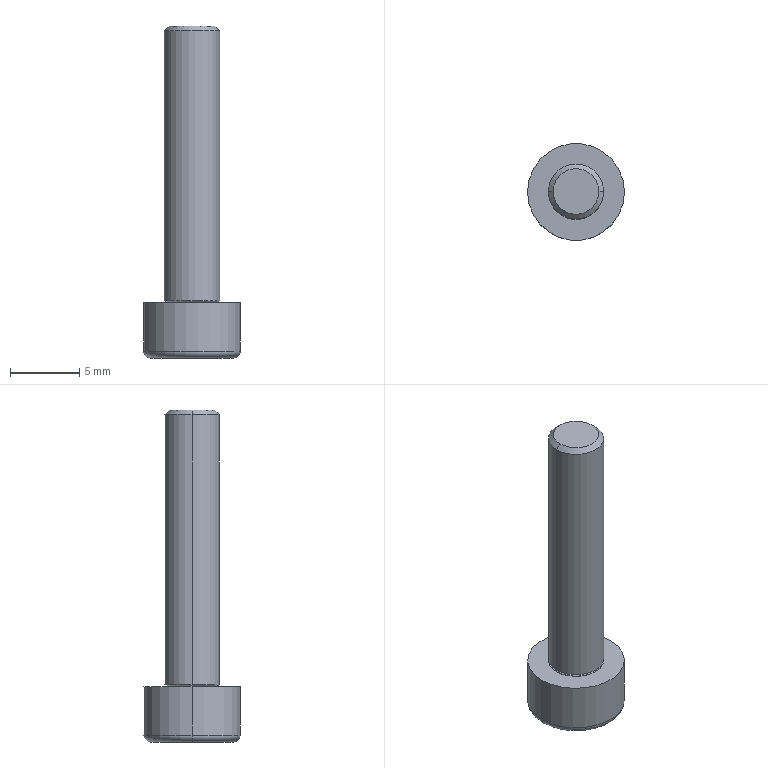Part | SolidWorks | features BaseBody 1 | 1 solid | 27 faces | box 7 x 7 x 24 mm | volume 391.462 mm3 | plane 11 | torus 6 | cylinder 6 | cone 4 | commonest cylinder face diameters 4 x4 7 x2
STEP:
#1=CARTESIAN_POINT('',(-1.763,0.,0.01));
#2=VERTEX_POINT('',#1);
#3=CARTESIAN_POINT('',(-1.743,0.,0.03));
#4=VERTEX_POINT('',#3);
#5=CARTESIAN_POINT('',(-1.763,0.,0.03));
#6=DIRECTION('',(0.,-1.,0.));
#7=DIRECTION('',(0.,0.,-1.));
#8=AXIS2_PLACEMENT_3D('',#5,#6,#7);
#9=CIRCLE('',#8,0.02);
#10=EDGE_CURVE('',#2,#4,#9,.T.);
#11=ORIENTED_EDGE('',*,*,#10,.T.);
#12=CARTESIAN_POINT('',(1.743,0.,0.03));
#13=VERTEX_POINT('',#12);
#14=CARTESIAN_POINT('',(0.,0.,0.03));
#15=DIRECTION('',(0.,0.,-1.));
#16=DIRECTION('',(-1.,0.,0.));
#17=AXIS2_PLACEMENT_3D('',#14,#15,#16);
#18=CIRCLE('',#17,1.743);
#19=EDGE_CURVE('',#4,#13,#18,.T.);
#20=ORIENTED_EDGE('',*,*,#19,.T.);
#21=CARTESIAN_POINT('',(1.763,0.,0.01));
#22=VERTEX_POINT('',#21);
#23=CARTESIAN_POINT('',(1.763,0.,0.03));
#24=DIRECTION('',(0.,1.,0.));
#25=DIRECTION('',(-1.,0.,0.));
#26=AXIS2_PLACEMENT_3D('',#23,#24,#25);
#27=CIRCLE('',#26,0.02);
#28=EDGE_CURVE('',#22,#13,#27,.T.);
#29=ORIENTED_EDGE('',*,*,#28,.F.);
#30=CARTESIAN_POINT('',(0.,0.,0.01));
#31=DIRECTION('',(0.,0.,-1.));
#32=DIRECTION('',(-1.,0.,0.));
#33=AXIS2_PLACEMENT_3D('',#30,#31,#32);
#34=CIRCLE('',#33,1.763);
#35=EDGE_CURVE('',#2,#22,#34,.T.);
#36=ORIENTED_EDGE('',*,*,#35,.F.);
#37=EDGE_LOOP('',(#11,#20,#29,#36));
#38=FACE_OUTER_BOUND('',#37,.T.);
#39=CARTESIAN_POINT('',(0.,0.,0.03));
#40=DIRECTION('',(0.,0.,-1.));
#41=DIRECTION('',(-1.,0.,0.));
#42=AXIS2_PLACEMENT_3D('',#39,#40,#41);
#43=TOROIDAL_SURFACE('',#42,1.763,0.02);
#44=ADVANCED_FACE('',(#38),#43,.F.);
#45=ORIENTED_EDGE('',*,*,#28,.T.);
#46=CARTESIAN_POINT('',(0.,0.,0.03));
#47=DIRECTION('',(0.,0.,-1.));
#48=DIRECTION('',(-1.,0.,0.));
#49=AXIS2_PLACEMENT_3D('',#46,#47,#48);
#50=CIRCLE('',#49,1.743);
#51=EDGE_CURVE('',#13,#4,#50,.T.);
#52=ORIENTED_EDGE('',*,*,#51,.T.);
#53=ORIENTED_EDGE('',*,*,#10,.F.);
#54=CARTESIAN_POINT('',(0.,0.,0.01));
#55=DIRECTION('',(0.,0.,-1.));
#56=DIRECTION('',(-1.,0.,0.));
#57=AXIS2_PLACEMENT_3D('',#54,#55,#56);
#58=CIRCLE('',#57,1.763);
#59=EDGE_CURVE('',#22,#2,#58,.T.);
#60=ORIENTED_EDGE('',*,*,#59,.F.);
#61=EDGE_LOOP('',(#45,#52,#53,#60));
#62=FACE_OUTER_BOUND('',#61,.T.);
#63=CARTESIAN_POINT('',(0.,0.,0.03));
#64=DIRECTION('',(0.,0.,-1.));
#65=DIRECTION('',(-1.,0.,0.));
#66=AXIS2_PLACEMENT_3D('',#63,#64,#65);
#67=TOROIDAL_SURFACE('',#66,1.763,0.02);
#68=ADVANCED_FACE('',(#62),#67,.F.);
#69=CARTESIAN_POINT('',(-1.65,0.,20.));
#70=VERTEX_POINT('',#69);
#71=CARTESIAN_POINT('',(1.65,0.,20.));
#72=VERTEX_POINT('',#71);
#73=CARTESIAN_POINT('',(0.,0.,20.));
#74=DIRECTION('',(0.,0.,-1.));
#75=DIRECTION('',(-1.,0.,0.));
#76=AXIS2_PLACEMENT_3D('',#73,#74,#75);
#77=CIRCLE('',#76,1.65);
#78=EDGE_CURVE('',#70,#72,#77,.T.);
#79=ORIENTED_EDGE('',*,*,#78,.T.);
#80=CARTESIAN_POINT('',(2.,0.,19.65));
#81=VERTEX_POINT('',#80);
#82=CARTESIAN_POINT('',(1.65,0.,20.));
#83=DIRECTION('',(0.7071,0.,-0.7071));
#84=VECTOR('',#83,1000.);
#85=LINE('',#82,#84);
#86=EDGE_CURVE('',#72,#81,#85,.T.);
#87=ORIENTED_EDGE('',*,*,#86,.T.);
#88=CARTESIAN_POINT('',(-2.,0.,19.65));
#89=VERTEX_POINT('',#88);
#90=CARTESIAN_POINT('',(0.,0.,19.65));
#91=DIRECTION('',(0.,0.,-1.));
#92=DIRECTION('',(-1.,0.,0.));
#93=AXIS2_PLACEMENT_3D('',#90,#91,#92);
#94=CIRCLE('',#93,2.);
#95=EDGE_CURVE('',#89,#81,#94,.T.);
#96=ORIENTED_EDGE('',*,*,#95,.F.);
#97=CARTESIAN_POINT('',(-1.65,0.,20.));
#98=DIRECTION('',(-0.7071,0.,-0.7071));
#99=VECTOR('',#98,1000.);
#100=LINE('',#97,#99);
#101=EDGE_CURVE('',#70,#89,#100,.T.);
#102=ORIENTED_EDGE('',*,*,#101,.F.);
#103=EDGE_LOOP('',(#79,#87,#96,#102));
#104=FACE_OUTER_BOUND('',#103,.T.);
#105=CARTESIAN_POINT('',(0.,0.,20.));
#106=DIRECTION('',(0.,0.,-1.));
#107=DIRECTION('',(-1.,0.,0.));
#108=AXIS2_PLACEMENT_3D('',#105,#106,#107);
#109=CONICAL_SURFACE('',#108,1.65,0.7854);
#110=ADVANCED_FACE('',(#104),#109,.T.);
#111=ORIENTED_EDGE('',*,*,#95,.T.);
#112=CARTESIAN_POINT('',(2.,0.,0.1374));
#113=VERTEX_POINT('',#112);
#114=CARTESIAN_POINT('',(2.,0.,-10.585));
#115=DIRECTION('',(0.,0.,-1.));
#116=VECTOR('',#115,1000.);
#117=LINE('',#114,#116);
#118=EDGE_CURVE('',#81,#113,#117,.T.);
#119=ORIENTED_EDGE('',*,*,#118,.T.);
#120=CARTESIAN_POINT('',(-2.,0.,0.1374));
#121=VERTEX_POINT('',#120);
#122=CARTESIAN_POINT('',(0.,0.,0.1374));
#123=DIRECTION('',(0.,0.,-1.));
#124=DIRECTION('',(-1.,0.,0.));
#125=AXIS2_PLACEMENT_3D('',#122,#123,#124);
#126=CIRCLE('',#125,2.);
#127=EDGE_CURVE('',#121,#113,#126,.T.);
#128=ORIENTED_EDGE('',*,*,#127,.F.);
#129=CARTESIAN_POINT('',(-2.,0.,-10.585));
#130=DIRECTION('',(0.,0.,-1.));
#131=VECTOR('',#130,1000.);
#132=LINE('',#129,#131);
#133=EDGE_CURVE('',#89,#121,#132,.T.);
#134=ORIENTED_EDGE('',*,*,#133,.F.);
#135=EDGE_LOOP('',(#111,#119,#128,#134));
#136=FACE_OUTER_BOUND('',#135,.T.);
#137=CARTESIAN_POINT('',(0.,0.,-10.585));
#138=DIRECTION('',(0.,0.,-1.));
#139=DIRECTION('',(-1.,0.,0.));
#140=AXIS2_PLACEMENT_3D('',#137,#138,#139);
#141=CYLINDRICAL_SURFACE('',#140,2.);
#142=ADVANCED_FACE('',(#136),#141,.T.);
#143=CARTESIAN_POINT('',(-1.757,0.,0.04879));
#144=VERTEX_POINT('',#143);
#145=CARTESIAN_POINT('',(1.757,0.,0.04879));
#146=VERTEX_POINT('',#145);
#147=CARTESIAN_POINT('',(0.,0.,0.04879));
#148=DIRECTION('',(0.,0.,-1.));
#149=DIRECTION('',(-1.,0.,0.));
#150=AXIS2_PLACEMENT_3D('',#147,#148,#149);
#151=CIRCLE('',#150,1.757);
#152=EDGE_CURVE('',#144,#146,#151,.T.);
#153=ORIENTED_EDGE('',*,*,#152,.F.);
#154=CARTESIAN_POINT('',(-2.,0.,0.1374));
#155=DIRECTION('',(-0.9397,0.,0.342));
#156=VECTOR('',#155,1000.);
#157=LINE('',#154,#156);
#158=EDGE_CURVE('',#144,#121,#157,.T.);
#159=ORIENTED_EDGE('',*,*,#158,.T.);
#160=ORIENTED_EDGE('',*,*,#127,.T.);
#161=CARTESIAN_POINT('',(2.,0.,0.1374));
#162=DIRECTION('',(0.9397,0.,0.342));
#163=VECTOR('',#162,1000.);
#164=LINE('',#161,#163);
#165=EDGE_CURVE('',#146,#113,#164,.T.);
#166=ORIENTED_EDGE('',*,*,#165,.F.);
#167=EDGE_LOOP('',(#153,#159,#160,#166));
#168=FACE_OUTER_BOUND('',#167,.T.);
#169=CARTESIAN_POINT('',(0.,0.,0.1374));
#170=DIRECTION('',(0.,0.,1.));
#171=DIRECTION('',(1.,0.,0.));
#172=AXIS2_PLACEMENT_3D('',#169,#170,#171);
#173=CONICAL_SURFACE('',#172,2.,1.222);
#174=ADVANCED_FACE('',(#168),#173,.T.);
#175=ORIENTED_EDGE('',*,*,#51,.F.);
#176=CARTESIAN_POINT('',(1.763,0.,0.03));
#177=DIRECTION('',(0.,1.,0.));
#178=DIRECTION('',(-1.,0.,0.));
#179=AXIS2_PLACEMENT_3D('',#176,#177,#178);
#180=CIRCLE('',#179,0.02);
#181=EDGE_CURVE('',#13,#146,#180,.T.);
#182=ORIENTED_EDGE('',*,*,#181,.T.);
#183=CARTESIAN_POINT('',(0.,0.,0.04879));
#184=DIRECTION('',(0.,0.,-1.));
#185=DIRECTION('',(-1.,0.,0.));
#186=AXIS2_PLACEMENT_3D('',#183,#184,#185);
#187=CIRCLE('',#186,1.757);
#188=EDGE_CURVE('',#146,#144,#187,.T.);
#189=ORIENTED_EDGE('',*,*,#188,.T.);
#190=CARTESIAN_POINT('',(-1.763,0.,0.03));
#191=DIRECTION('',(0.,-1.,0.));
#192=DIRECTION('',(0.,0.,-1.));
#193=AXIS2_PLACEMENT_3D('',#190,#191,#192);
#194=CIRCLE('',#193,0.02);
#195=EDGE_CURVE('',#4,#144,#194,.T.);
#196=ORIENTED_EDGE('',*,*,#195,.F.);
#197=EDGE_LOOP('',(#175,#182,#189,#196));
#198=FACE_OUTER_BOUND('',#197,.T.);
#199=CARTESIAN_POINT('',(0.,0.,0.03));
#200=DIRECTION('',(0.,0.,-1.));
#201=DIRECTION('',(-1.,0.,0.));
#202=AXIS2_PLACEMENT_3D('',#199,#200,#201);
#203=TOROIDAL_SURFACE('',#202,1.763,0.02);
#204=ADVANCED_FACE('',(#198),#203,.F.);
#205=CARTESIAN_POINT('',(-2.,0.,0.01));
#206=VERTEX_POINT('',#205);
#207=CARTESIAN_POINT('',(2.,0.,0.01));
#208=VERTEX_POINT('',#207);
#209=CARTESIAN_POINT('',(0.,0.,0.01));
#210=DIRECTION('',(0.,0.,-1.));
#211=DIRECTION('',(-1.,0.,0.));
#212=AXIS2_PLACEMENT_3D('',#209,#210,#211);
#213=CIRCLE('',#212,2.);
#214=EDGE_CURVE('',#206,#208,#213,.T.);
#215=ORIENTED_EDGE('',*,*,#214,.T.);
#216=CARTESIAN_POINT('',(2.,0.,0.));
#217=VERTEX_POINT('',#216);
#218=CARTESIAN_POINT('',(2.,0.,-10.585));
#219=DIRECTION('',(0.,0.,-1.));
#220=VECTOR('',#219,1000.);
#221=LINE('',#218,#220);
#222=EDGE_CURVE('',#208,#217,#221,.T.);
#223=ORIENTED_EDGE('',*,*,#222,.T.);
#224=CARTESIAN_POINT('',(-2.,0.,0.));
#225=VERTEX_POINT('',#224);
#226=CARTESIAN_POINT('',(0.,0.,0.));
#227=DIRECTION('',(0.,0.,-1.));
#228=DIRECTION('',(-1.,0.,0.));
#229=AXIS2_PLACEMENT_3D('',#226,#227,#228);
#230=CIRCLE('',#229,2.);
#231=EDGE_CURVE('',#225,#217,#230,.T.);
#232=ORIENTED_EDGE('',*,*,#231,.F.);
#233=CARTESIAN_POINT('',(-2.,0.,-10.585));
#234=DIRECTION('',(0.,0.,-1.));
#235=VECTOR('',#234,1000.);
#236=LINE('',#233,#235);
#237=EDGE_CURVE('',#206,#225,#236,.T.);
#238=ORIENTED_EDGE('',*,*,#237,.F.);
#239=EDGE_LOOP('',(#215,#223,#232,#238));
#240=FACE_OUTER_BOUND('',#239,.T.);
#241=CARTESIAN_POINT('',(0.,0.,-10.585));
#242=DIRECTION('',(0.,0.,-1.));
#243=DIRECTION('',(-1.,0.,0.));
#244=AXIS2_PLACEMENT_3D('',#241,#242,#243);
#245=CYLINDRICAL_SURFACE('',#244,2.);
#246=ADVANCED_FACE('',(#240),#245,.T.);
#247=CARTESIAN_POINT('',(-3.5,0.,0.));
#248=VERTEX_POINT('',#247);
#249=CARTESIAN_POINT('',(3.5,0.,0.));
#250=VERTEX_POINT('',#249);
#251=CARTESIAN_POINT('',(0.,0.,0.));
#252=DIRECTION('',(0.,0.,-1.));
#253=DIRECTION('',(-1.,0.,0.));
#254=AXIS2_PLACEMENT_3D('',#251,#252,#253);
#255=CIRCLE('',#254,3.5);
#256=EDGE_CURVE('',#248,#250,#255,.T.);
#257=ORIENTED_EDGE('',*,*,#256,.T.);
#258=CARTESIAN_POINT('',(3.5,0.,-3.5));
#259=VERTEX_POINT('',#258);
#260=CARTESIAN_POINT('',(3.5,0.,-10.585));
#261=DIRECTION('',(0.,0.,-1.));
#262=VECTOR('',#261,1000.);
#263=LINE('',#260,#262);
#264=EDGE_CURVE('',#250,#259,#263,.T.);
#265=ORIENTED_EDGE('',*,*,#264,.T.);
#266=CARTESIAN_POINT('',(-3.5,0.,-3.5));
#267=VERTEX_POINT('',#266);
#268=CARTESIAN_POINT('',(0.,0.,-3.5));
#269=DIRECTION('',(0.,0.,-1.));
#270=DIRECTION('',(-1.,0.,0.));
#271=AXIS2_PLACEMENT_3D('',#268,#269,#270);
#272=CIRCLE('',#271,3.5);
#273=EDGE_CURVE('',#267,#259,#272,.T.);
#274=ORIENTED_EDGE('',*,*,#273,.F.);
#275=CARTESIAN_POINT('',(-3.5,0.,-10.585));
#276=DIRECTION('',(0.,0.,-1.));
#277=VECTOR('',#276,1000.);
#278=LINE('',#275,#277);
#279=EDGE_CURVE('',#248,#267,#278,.T.);
#280=ORIENTED_EDGE('',*,*,#279,.F.);
#281=EDGE_LOOP('',(#257,#265,#274,#280));
#282=FACE_OUTER_BOUND('',#281,.T.);
#283=CARTESIAN_POINT('',(0.,0.,-10.585));
#284=DIRECTION('',(0.,0.,-1.));
#285=DIRECTION('',(-1.,0.,0.));
#286=AXIS2_PLACEMENT_3D('',#283,#284,#285);
#287=CYLINDRICAL_SURFACE('',#286,3.5);
#288=ADVANCED_FACE('',(#282),#287,.T.);
#289=ORIENTED_EDGE('',*,*,#273,.T.);
#290=CARTESIAN_POINT('',(3.,0.,-4.));
#291=VERTEX_POINT('',#290);
#292=CARTESIAN_POINT('',(3.,0.,-3.5));
#293=DIRECTION('',(0.,1.,0.));
#294=DIRECTION('',(-1.,0.,0.));
#295=AXIS2_PLACEMENT_3D('',#292,#293,#294);
#296=CIRCLE('',#295,0.5);
#297=EDGE_CURVE('',#259,#291,#296,.T.);
#298=ORIENTED_EDGE('',*,*,#297,.T.);
#299=CARTESIAN_POINT('',(-3.,0.,-4.));
#300=VERTEX_POINT('',#299);
#301=CARTESIAN_POINT('',(0.,0.,-4.));
#302=DIRECTION('',(0.,0.,-1.));
#303=DIRECTION('',(-1.,0.,0.));
#304=AXIS2_PLACEMENT_3D('',#301,#302,#303);
#305=CIRCLE('',#304,3.);
#306=EDGE_CURVE('',#300,#291,#305,.T.);
#307=ORIENTED_EDGE('',*,*,#306,.F.);
#308=CARTESIAN_POINT('',(-3.,0.,-3.5));
#309=DIRECTION('',(0.,-1.,0.));
#310=DIRECTION('',(0.,0.,-1.));
#311=AXIS2_PLACEMENT_3D('',#308,#309,#310);
#312=CIRCLE('',#311,0.5);
#313=EDGE_CURVE('',#267,#300,#312,.T.);
#314=ORIENTED_EDGE('',*,*,#313,.F.);
#315=EDGE_LOOP('',(#289,#298,#307,#314));
#316=FACE_OUTER_BOUND('',#315,.T.);
#317=CARTESIAN_POINT('',(0.,0.,-3.5));
#318=DIRECTION('',(0.,0.,-1.));
#319=DIRECTION('',(-1.,0.,0.));
#320=AXIS2_PLACEMENT_3D('',#317,#318,#319);
#321=TOROIDAL_SURFACE('',#320,3.,0.5);
#322=ADVANCED_FACE('',(#316),#321,.T.);
#323=ORIENTED_EDGE('',*,*,#297,.F.);
#324=CARTESIAN_POINT('',(0.,0.,-3.5));
#325=DIRECTION('',(0.,0.,-1.));
#326=DIRECTION('',(-1.,0.,0.));
#327=AXIS2_PLACEMENT_3D('',#324,#325,#326);
#328=CIRCLE('',#327,3.5);
#329=EDGE_CURVE('',#259,#267,#328,.T.);
#330=ORIENTED_EDGE('',*,*,#329,.T.);
#331=ORIENTED_EDGE('',*,*,#313,.T.);
#332=CARTESIAN_POINT('',(0.,0.,-4.));
#333=DIRECTION('',(0.,0.,-1.));
#334=DIRECTION('',(-1.,0.,0.));
#335=AXIS2_PLACEMENT_3D('',#332,#333,#334);
#336=CIRCLE('',#335,3.);
#337=EDGE_CURVE('',#291,#300,#336,.T.);
#338=ORIENTED_EDGE('',*,*,#337,.F.);
#339=EDGE_LOOP('',(#323,#330,#331,#338));
#340=FACE_OUTER_BOUND('',#339,.T.);
#341=CARTESIAN_POINT('',(0.,0.,-3.5));
#342=DIRECTION('',(0.,0.,-1.));
#343=DIRECTION('',(-1.,0.,0.));
#344=AXIS2_PLACEMENT_3D('',#341,#342,#343);
#345=TOROIDAL_SURFACE('',#344,3.,0.5);
#346=ADVANCED_FACE('',(#340),#345,.T.);
#347=ORIENTED_EDGE('',*,*,#264,.F.);
#348=CARTESIAN_POINT('',(0.,0.,0.));
#349=DIRECTION('',(0.,0.,-1.));
#350=DIRECTION('',(-1.,0.,0.));
#351=AXIS2_PLACEMENT_3D('',#348,#349,#350);
#352=CIRCLE('',#351,3.5);
#353=EDGE_CURVE('',#250,#248,#352,.T.);
#354=ORIENTED_EDGE('',*,*,#353,.T.);
#355=ORIENTED_EDGE('',*,*,#279,.T.);
#356=ORIENTED_EDGE('',*,*,#329,.F.);
#357=EDGE_LOOP('',(#347,#354,#355,#356));
#358=FACE_OUTER_BOUND('',#357,.T.);
#359=CARTESIAN_POINT('',(0.,0.,-10.585));
#360=DIRECTION('',(0.,0.,-1.));
#361=DIRECTION('',(-1.,0.,0.));
#362=AXIS2_PLACEMENT_3D('',#359,#360,#361);
#363=CYLINDRICAL_SURFACE('',#362,3.5);
#364=ADVANCED_FACE('',(#358),#363,.T.);
#365=ORIENTED_EDGE('',*,*,#256,.F.);
#366=ORIENTED_EDGE('',*,*,#353,.F.);
#367=EDGE_LOOP('',(#365,#366));
#368=FACE_OUTER_BOUND('',#367,.T.);
#369=ORIENTED_EDGE('',*,*,#231,.T.);
#370=CARTESIAN_POINT('',(0.,0.,0.));
#371=DIRECTION('',(0.,0.,-1.));
#372=DIRECTION('',(-1.,0.,0.));
#373=AXIS2_PLACEMENT_3D('',#370,#371,#372);
#374=CIRCLE('',#373,2.);
#375=EDGE_CURVE('',#217,#225,#374,.T.);
#376=ORIENTED_EDGE('',*,*,#375,.T.);
#377=EDGE_LOOP('',(#369,#376));
#378=FACE_BOUND('',#377,.T.);
#379=CARTESIAN_POINT('',(-3.5,0.,0.));
#380=DIRECTION('',(0.,0.,-1.));
#381=DIRECTION('',(-1.,0.,0.));
#382=AXIS2_PLACEMENT_3D('',#379,#380,#381);
#383=PLANE('',#382);
#384=ADVANCED_FACE('',(#368,#378),#383,.F.);
#385=ORIENTED_EDGE('',*,*,#222,.F.);
#386=CARTESIAN_POINT('',(0.,0.,0.01));
#387=DIRECTION('',(0.,0.,-1.));
#388=DIRECTION('',(-1.,0.,0.));
#389=AXIS2_PLACEMENT_3D('',#386,#387,#388);
#390=CIRCLE('',#389,2.);
#391=EDGE_CURVE('',#208,#206,#390,.T.);
#392=ORIENTED_EDGE('',*,*,#391,.T.);
#393=ORIENTED_EDGE('',*,*,#237,.T.);
#394=ORIENTED_EDGE('',*,*,#375,.F.);
#395=EDGE_LOOP('',(#385,#392,#393,#394));
#396=FACE_OUTER_BOUND('',#395,.T.);
#397=CARTESIAN_POINT('',(0.,0.,-10.585));
#398=DIRECTION('',(0.,0.,-1.));
#399=DIRECTION('',(-1.,0.,0.));
#400=AXIS2_PLACEMENT_3D('',#397,#398,#399);
#401=CYLINDRICAL_SURFACE('',#400,2.);
#402=ADVANCED_FACE('',(#396),#401,.T.);
#403=ORIENTED_EDGE('',*,*,#214,.F.);
#404=ORIENTED_EDGE('',*,*,#391,.F.);
#405=EDGE_LOOP('',(#403,#404));
#406=FACE_OUTER_BOUND('',#405,.T.);
#407=ORIENTED_EDGE('',*,*,#35,.T.);
#408=ORIENTED_EDGE('',*,*,#59,.T.);
#409=EDGE_LOOP('',(#407,#408));
#410=FACE_BOUND('',#409,.T.);
#411=CARTESIAN_POINT('',(-2.,0.,0.01));
#412=DIRECTION('',(0.,0.,-1.));
#413=DIRECTION('',(-1.,0.,0.));
#414=AXIS2_PLACEMENT_3D('',#411,#412,#413);
#415=PLANE('',#414);
#416=ADVANCED_FACE('',(#406,#410),#415,.F.);
#417=ORIENTED_EDGE('',*,*,#19,.F.);
#418=ORIENTED_EDGE('',*,*,#195,.T.);
#419=ORIENTED_EDGE('',*,*,#152,.T.);
#420=ORIENTED_EDGE('',*,*,#181,.F.);
#421=EDGE_LOOP('',(#417,#418,#419,#420));
#422=FACE_OUTER_BOUND('',#421,.T.);
#423=CARTESIAN_POINT('',(0.,0.,0.03));
#424=DIRECTION('',(0.,0.,-1.));
#425=DIRECTION('',(-1.,0.,0.));
#426=AXIS2_PLACEMENT_3D('',#423,#424,#425);
#427=TOROIDAL_SURFACE('',#426,1.763,0.02);
#428=ADVANCED_FACE('',(#422),#427,.F.);
#429=ORIENTED_EDGE('',*,*,#158,.F.);
#430=ORIENTED_EDGE('',*,*,#188,.F.);
#431=ORIENTED_EDGE('',*,*,#165,.T.);
#432=CARTESIAN_POINT('',(0.,0.,0.1374));
#433=DIRECTION('',(0.,0.,-1.));
#434=DIRECTION('',(-1.,0.,0.));
#435=AXIS2_PLACEMENT_3D('',#432,#433,#434);
#436=CIRCLE('',#435,2.);
#437=EDGE_CURVE('',#113,#121,#436,.T.);
#438=ORIENTED_EDGE('',*,*,#437,.T.);
#439=EDGE_LOOP('',(#429,#430,#431,#438));
#440=FACE_OUTER_BOUND('',#439,.T.);
#441=CARTESIAN_POINT('',(0.,0.,0.1374));
#442=DIRECTION('',(0.,0.,1.));
#443=DIRECTION('',(1.,0.,0.));
#444=AXIS2_PLACEMENT_3D('',#441,#442,#443);
#445=CONICAL_SURFACE('',#444,2.,1.222);
#446=ADVANCED_FACE('',(#440),#445,.T.);
#447=ORIENTED_EDGE('',*,*,#118,.F.);
#448=CARTESIAN_POINT('',(0.,0.,19.65));
#449=DIRECTION('',(0.,0.,-1.));
#450=DIRECTION('',(-1.,0.,0.));
#451=AXIS2_PLACEMENT_3D('',#448,#449,#450);
#452=CIRCLE('',#451,2.);
#453=EDGE_CURVE('',#81,#89,#452,.T.);
#454=ORIENTED_EDGE('',*,*,#453,.T.);
#455=ORIENTED_EDGE('',*,*,#133,.T.);
#456=ORIENTED_EDGE('',*,*,#437,.F.);
#457=EDGE_LOOP('',(#447,#454,#455,#456));
#458=FACE_OUTER_BOUND('',#457,.T.);
#459=CARTESIAN_POINT('',(0.,0.,-10.585));
#460=DIRECTION('',(0.,0.,-1.));
#461=DIRECTION('',(-1.,0.,0.));
#462=AXIS2_PLACEMENT_3D('',#459,#460,#461);
#463=CYLINDRICAL_SURFACE('',#462,2.);
#464=ADVANCED_FACE('',(#458),#463,.T.);
#465=ORIENTED_EDGE('',*,*,#86,.F.);
#466=CARTESIAN_POINT('',(0.,0.,20.));
#467=DIRECTION('',(0.,0.,-1.));
#468=DIRECTION('',(-1.,0.,0.));
#469=AXIS2_PLACEMENT_3D('',#466,#467,#468);
#470=CIRCLE('',#469,1.65);
#471=EDGE_CURVE('',#72,#70,#470,.T.);
#472=ORIENTED_EDGE('',*,*,#471,.T.);
#473=ORIENTED_EDGE('',*,*,#101,.T.);
#474=ORIENTED_EDGE('',*,*,#453,.F.);
#475=EDGE_LOOP('',(#465,#472,#473,#474));
#476=FACE_OUTER_BOUND('',#475,.T.);
#477=CARTESIAN_POINT('',(0.,0.,20.));
#478=DIRECTION('',(0.,0.,-1.));
#479=DIRECTION('',(-1.,0.,0.));
#480=AXIS2_PLACEMENT_3D('',#477,#478,#479);
#481=CONICAL_SURFACE('',#480,1.65,0.7854);
#482=ADVANCED_FACE('',(#476),#481,.T.);
#483=ORIENTED_EDGE('',*,*,#78,.F.);
#484=ORIENTED_EDGE('',*,*,#471,.F.);
#485=EDGE_LOOP('',(#483,#484));
#486=FACE_OUTER_BOUND('',#485,.T.);
#487=CARTESIAN_POINT('',(-1.65,0.,20.));
#488=DIRECTION('',(0.,0.,-1.));
#489=DIRECTION('',(-1.,0.,0.));
#490=AXIS2_PLACEMENT_3D('',#487,#488,#489);
#491=PLANE('',#490);
#492=ADVANCED_FACE('',(#486),#491,.F.);
#493=CARTESIAN_POINT('',(1.732,0.,-4.));
#494=VERTEX_POINT('',#493);
#495=CARTESIAN_POINT('',(0.866,-1.5,-4.));
#496=VERTEX_POINT('',#495);
#497=CARTESIAN_POINT('',(1.732,0.,-4.));
#498=DIRECTION('',(-0.5,-0.866,0.));
#499=VECTOR('',#498,1000.);
#500=LINE('',#497,#499);
#501=EDGE_CURVE('',#494,#496,#500,.T.);
#502=ORIENTED_EDGE('',*,*,#501,.F.);
#503=CARTESIAN_POINT('',(0.866,1.5,-4.));
#504=VERTEX_POINT('',#503);
#505=CARTESIAN_POINT('',(0.866,1.5,-4.));
#506=DIRECTION('',(0.5,-0.866,0.));
#507=VECTOR('',#506,1000.);
#508=LINE('',#505,#507);
#509=EDGE_CURVE('',#504,#494,#508,.T.);
#510=ORIENTED_EDGE('',*,*,#509,.F.);
#511=CARTESIAN_POINT('',(-0.866,1.5,-4.));
#512=VERTEX_POINT('',#511);
#513=CARTESIAN_POINT('',(-0.866,1.5,-4.));
#514=DIRECTION('',(1.,0.,0.));
#515=VECTOR('',#514,1000.);
#516=LINE('',#513,#515);
#517=EDGE_CURVE('',#512,#504,#516,.T.);
#518=ORIENTED_EDGE('',*,*,#517,.F.);
#519=CARTESIAN_POINT('',(-1.732,0.,-4.));
#520=VERTEX_POINT('',#519);
#521=CARTESIAN_POINT('',(-1.732,0.,-4.));
#522=DIRECTION('',(0.5,0.866,0.));
#523=VECTOR('',#522,1000.);
#524=LINE('',#521,#523);
#525=EDGE_CURVE('',#520,#512,#524,.T.);
#526=ORIENTED_EDGE('',*,*,#525,.F.);
#527=CARTESIAN_POINT('',(-0.866,-1.5,-4.));
#528=VERTEX_POINT('',#527);
#529=CARTESIAN_POINT('',(-0.866,-1.5,-4.));
#530=DIRECTION('',(-0.5,0.866,0.));
#531=VECTOR('',#530,1000.);
#532=LINE('',#529,#531);
#533=EDGE_CURVE('',#528,#520,#532,.T.);
#534=ORIENTED_EDGE('',*,*,#533,.F.);
#535=CARTESIAN_POINT('',(0.866,-1.5,-4.));
#536=DIRECTION('',(-1.,0.,0.));
#537=VECTOR('',#536,1000.);
#538=LINE('',#535,#537);
#539=EDGE_CURVE('',#496,#528,#538,.T.);
#540=ORIENTED_EDGE('',*,*,#539,.F.);
#541=EDGE_LOOP('',(#502,#510,#518,#526,#534,#540));
#542=FACE_BOUND('',#541,.T.);
#543=ORIENTED_EDGE('',*,*,#306,.T.);
#544=ORIENTED_EDGE('',*,*,#337,.T.);
#545=EDGE_LOOP('',(#543,#544));
#546=FACE_OUTER_BOUND('',#545,.T.);
#547=CARTESIAN_POINT('',(0.,0.,-4.));
#548=DIRECTION('',(0.,0.,1.));
#549=DIRECTION('',(1.,0.,0.));
#550=AXIS2_PLACEMENT_3D('',#547,#548,#549);
#551=PLANE('',#550);
#552=ADVANCED_FACE('',(#542,#546),#551,.F.);
#553=ORIENTED_EDGE('',*,*,#509,.T.);
#554=CARTESIAN_POINT('',(1.732,0.,-2.5));
#555=VERTEX_POINT('',#554);
#556=CARTESIAN_POINT('',(1.732,0.,-2.5));
#557=DIRECTION('',(0.,0.,-1.));
#558=VECTOR('',#557,1000.);
#559=LINE('',#556,#558);
#560=EDGE_CURVE('',#555,#494,#559,.T.);
#561=ORIENTED_EDGE('',*,*,#560,.F.);
#562=CARTESIAN_POINT('',(0.866,1.5,-2.5));
#563=VERTEX_POINT('',#562);
#564=CARTESIAN_POINT('',(0.866,1.5,-2.5));
#565=DIRECTION('',(0.5,-0.866,0.));
#566=VECTOR('',#565,1000.);
#567=LINE('',#564,#566);
#568=EDGE_CURVE('',#563,#555,#567,.T.);
#569=ORIENTED_EDGE('',*,*,#568,.F.);
#570=CARTESIAN_POINT('',(0.866,1.5,-2.5));
#571=DIRECTION('',(0.,0.,-1.));
#572=VECTOR('',#571,1000.);
#573=LINE('',#570,#572);
#574=EDGE_CURVE('',#563,#504,#573,.T.);
#575=ORIENTED_EDGE('',*,*,#574,.T.);
#576=EDGE_LOOP('',(#553,#561,#569,#575));
#577=FACE_OUTER_BOUND('',#576,.T.);
#578=CARTESIAN_POINT('',(0.866,1.5,-2.5));
#579=DIRECTION('',(0.866,0.5,0.));
#580=DIRECTION('',(-0.5,0.866,0.));
#581=AXIS2_PLACEMENT_3D('',#578,#579,#580);
#582=PLANE('',#581);
#583=ADVANCED_FACE('',(#577),#582,.F.);
#584=ORIENTED_EDGE('',*,*,#517,.T.);
#585=ORIENTED_EDGE('',*,*,#574,.F.);
#586=CARTESIAN_POINT('',(-0.866,1.5,-2.5));
#587=VERTEX_POINT('',#586);
#588=CARTESIAN_POINT('',(-0.866,1.5,-2.5));
#589=DIRECTION('',(1.,0.,0.));
#590=VECTOR('',#589,1000.);
#591=LINE('',#588,#590);
#592=EDGE_CURVE('',#587,#563,#591,.T.);
#593=ORIENTED_EDGE('',*,*,#592,.F.);
#594=CARTESIAN_POINT('',(-0.866,1.5,-2.5));
#595=DIRECTION('',(0.,0.,-1.));
#596=VECTOR('',#595,1000.);
#597=LINE('',#594,#596);
#598=EDGE_CURVE('',#587,#512,#597,.T.);
#599=ORIENTED_EDGE('',*,*,#598,.T.);
#600=EDGE_LOOP('',(#584,#585,#593,#599));
#601=FACE_OUTER_BOUND('',#600,.T.);
#602=CARTESIAN_POINT('',(-0.866,1.5,-2.5));
#603=DIRECTION('',(0.,1.,0.));
#604=DIRECTION('',(0.,0.,1.));
#605=AXIS2_PLACEMENT_3D('',#602,#603,#604);
#606=PLANE('',#605);
#607=ADVANCED_FACE('',(#601),#606,.F.);
#608=ORIENTED_EDGE('',*,*,#525,.T.);
#609=ORIENTED_EDGE('',*,*,#598,.F.);
#610=CARTESIAN_POINT('',(-1.732,0.,-2.5));
#611=VERTEX_POINT('',#610);
#612=CARTESIAN_POINT('',(-1.732,0.,-2.5));
#613=DIRECTION('',(0.5,0.866,0.));
#614=VECTOR('',#613,1000.);
#615=LINE('',#612,#614);
#616=EDGE_CURVE('',#611,#587,#615,.T.);
#617=ORIENTED_EDGE('',*,*,#616,.F.);
#618=CARTESIAN_POINT('',(-1.732,0.,-2.5));
#619=DIRECTION('',(0.,0.,-1.));
#620=VECTOR('',#619,1000.);
#621=LINE('',#618,#620);
#622=EDGE_CURVE('',#611,#520,#621,.T.);
#623=ORIENTED_EDGE('',*,*,#622,.T.);
#624=EDGE_LOOP('',(#608,#609,#617,#623));
#625=FACE_OUTER_BOUND('',#624,.T.);
#626=CARTESIAN_POINT('',(-1.732,0.,-2.5));
#627=DIRECTION('',(-0.866,0.5,0.));
#628=DIRECTION('',(-0.5,-0.866,0.));
#629=AXIS2_PLACEMENT_3D('',#626,#627,#628);
#630=PLANE('',#629);
#631=ADVANCED_FACE('',(#625),#630,.F.);
#632=ORIENTED_EDGE('',*,*,#533,.T.);
#633=ORIENTED_EDGE('',*,*,#622,.F.);
#634=CARTESIAN_POINT('',(-0.866,-1.5,-2.5));
#635=VERTEX_POINT('',#634);
#636=CARTESIAN_POINT('',(-0.866,-1.5,-2.5));
#637=DIRECTION('',(-0.5,0.866,0.));
#638=VECTOR('',#637,1000.);
#639=LINE('',#636,#638);
#640=EDGE_CURVE('',#635,#611,#639,.T.);
#641=ORIENTED_EDGE('',*,*,#640,.F.);
#642=CARTESIAN_POINT('',(-0.866,-1.5,-2.5));
#643=DIRECTION('',(0.,0.,-1.));
#644=VECTOR('',#643,1000.);
#645=LINE('',#642,#644);
#646=EDGE_CURVE('',#635,#528,#645,.T.);
#647=ORIENTED_EDGE('',*,*,#646,.T.);
#648=EDGE_LOOP('',(#632,#633,#641,#647));
#649=FACE_OUTER_BOUND('',#648,.T.);
#650=CARTESIAN_POINT('',(-0.866,-1.5,-2.5));
#651=DIRECTION('',(-0.866,-0.5,0.));
#652=DIRECTION('',(0.5,-0.866,0.));
#653=AXIS2_PLACEMENT_3D('',#650,#651,#652);
#654=PLANE('',#653);
#655=ADVANCED_FACE('',(#649),#654,.F.);
#656=ORIENTED_EDGE('',*,*,#539,.T.);
#657=ORIENTED_EDGE('',*,*,#646,.F.);
#658=CARTESIAN_POINT('',(0.866,-1.5,-2.5));
#659=VERTEX_POINT('',#658);
#660=CARTESIAN_POINT('',(0.866,-1.5,-2.5));
#661=DIRECTION('',(-1.,0.,0.));
#662=VECTOR('',#661,1000.);
#663=LINE('',#660,#662);
#664=EDGE_CURVE('',#659,#635,#663,.T.);
#665=ORIENTED_EDGE('',*,*,#664,.F.);
#666=CARTESIAN_POINT('',(0.866,-1.5,-2.5));
#667=DIRECTION('',(0.,0.,-1.));
#668=VECTOR('',#667,1000.);
#669=LINE('',#666,#668);
#670=EDGE_CURVE('',#659,#496,#669,.T.);
#671=ORIENTED_EDGE('',*,*,#670,.T.);
#672=EDGE_LOOP('',(#656,#657,#665,#671));
#673=FACE_OUTER_BOUND('',#672,.T.);
#674=CARTESIAN_POINT('',(0.866,-1.5,-2.5));
#675=DIRECTION('',(0.,-1.,0.));
#676=DIRECTION('',(0.,0.,-1.));
#677=AXIS2_PLACEMENT_3D('',#674,#675,#676);
#678=PLANE('',#677);
#679=ADVANCED_FACE('',(#673),#678,.F.);
#680=ORIENTED_EDGE('',*,*,#501,.T.);
#681=ORIENTED_EDGE('',*,*,#670,.F.);
#682=CARTESIAN_POINT('',(1.732,0.,-2.5));
#683=DIRECTION('',(-0.5,-0.866,0.));
#684=VECTOR('',#683,1000.);
#685=LINE('',#682,#684);
#686=EDGE_CURVE('',#555,#659,#685,.T.);
#687=ORIENTED_EDGE('',*,*,#686,.F.);
#688=ORIENTED_EDGE('',*,*,#560,.T.);
#689=EDGE_LOOP('',(#680,#681,#687,#688));
#690=FACE_OUTER_BOUND('',#689,.T.);
#691=CARTESIAN_POINT('',(1.732,0.,-2.5));
#692=DIRECTION('',(0.866,-0.5,0.));
#693=DIRECTION('',(0.5,0.866,0.));
#694=AXIS2_PLACEMENT_3D('',#691,#692,#693);
#695=PLANE('',#694);
#696=ADVANCED_FACE('',(#690),#695,.F.);
#697=ORIENTED_EDGE('',*,*,#568,.T.);
#698=ORIENTED_EDGE('',*,*,#686,.T.);
#699=ORIENTED_EDGE('',*,*,#664,.T.);
#700=ORIENTED_EDGE('',*,*,#640,.T.);
#701=ORIENTED_EDGE('',*,*,#616,.T.);
#702=ORIENTED_EDGE('',*,*,#592,.T.);
#703=EDGE_LOOP('',(#697,#698,#699,#700,#701,#702));
#704=FACE_OUTER_BOUND('',#703,.T.);
#705=CARTESIAN_POINT('',(0.866,1.5,-2.5));
#706=DIRECTION('',(0.,0.,1.));
#707=DIRECTION('',(1.,0.,0.));
#708=AXIS2_PLACEMENT_3D('',#705,#706,#707);
#709=PLANE('',#708);
#710=ADVANCED_FACE('',(#704),#709,.F.);
#711=CLOSED_SHELL('',(#44,#68,#110,#142,#174,#204,#246,#288,#322,#346,#364,#384,#402,#416,#428,#446,#464,#482,#492,#552,#583,#607,#631,#655,#679,#696,#710));
#712=MANIFOLD_SOLID_BREP('',#711);
#713=CARTESIAN_POINT('',(0.,0.,0.));
#714=DIRECTION('',(0.,0.,1.));
#715=DIRECTION('',(1.,0.,0.));
#716=AXIS2_PLACEMENT_3D('',#713,#714,#715);
#717=(LENGTH_UNIT()NAMED_UNIT(*)SI_UNIT(.MILLI.,.METRE.));
#718=UNCERTAINTY_MEASURE_WITH_UNIT(LENGTH_MEASURE(0.00001),#717,'','');
#719=(NAMED_UNIT(*)PLANE_ANGLE_UNIT()SI_UNIT($,.RADIAN.));
#720=(NAMED_UNIT(*)SI_UNIT($,.STERADIAN.)SOLID_ANGLE_UNIT());
#721=(GEOMETRIC_REPRESENTATION_CONTEXT(3)GLOBAL_UNCERTAINTY_ASSIGNED_CONTEXT((#718))GLOBAL_UNIT_ASSIGNED_CONTEXT((#717,#719,#720))REPRESENTATION_CONTEXT('',''));
#722=ADVANCED_BREP_SHAPE_REPRESENTATION('',(#712,#716),#721);